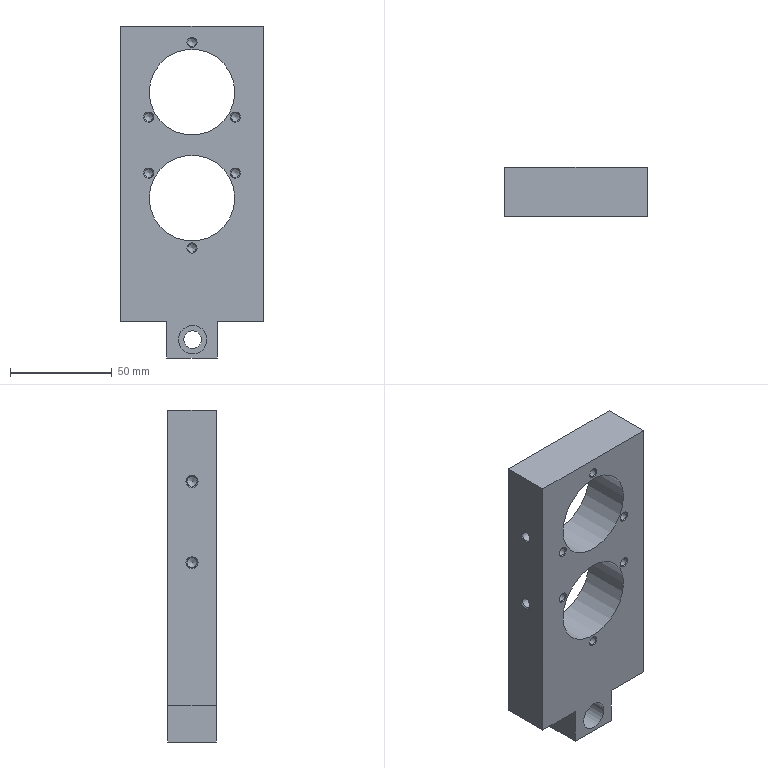Part | STEP file | 冲床-300配套压波_id346_x_t | 1 solid | 45 faces | box 70 x 24 x 163 mm | volume 181383 mm3 | cone 20 | cylinder 14 | plane 11 | commonest cylinder face diameters 4.2 x6 5 x2 8.5 x2 42 x2 8.7 x1 14 x1
STEP:
#1=CARTESIAN_POINT('',(1620.325,-84.,6.65));
#2=VERTEX_POINT('',#1);
#3=CARTESIAN_POINT('',(1620.325,-84.,11.));
#4=DIRECTION('',(0.,-1.,0.));
#5=DIRECTION('',(0.,0.,-1.));
#6=AXIS2_PLACEMENT_3D('',#3,#4,#5);
#7=CIRCLE('',#6,4.35);
#8=EDGE_CURVE('',#2,#2,#7,.T.);
#9=ORIENTED_EDGE('',*,*,#8,.F.);
#10=EDGE_LOOP('',(#9));
#11=FACE_BOUND('',#10,.T.);
#12=CARTESIAN_POINT('',(1620.325,-84.,4.));
#13=VERTEX_POINT('',#12);
#14=CARTESIAN_POINT('',(1620.325,-84.,11.));
#15=DIRECTION('',(0.,-1.,0.));
#16=DIRECTION('',(0.,0.,-1.));
#17=AXIS2_PLACEMENT_3D('',#14,#15,#16);
#18=CIRCLE('',#17,7.);
#19=EDGE_CURVE('',#13,#13,#18,.T.);
#20=ORIENTED_EDGE('',*,*,#19,.T.);
#21=EDGE_LOOP('',(#20));
#22=FACE_BOUND('',#21,.T.);
#23=CARTESIAN_POINT('',(1620.325,-84.,11.));
#24=DIRECTION('',(0.,1.,0.));
#25=DIRECTION('',(0.,0.,-1.));
#26=AXIS2_PLACEMENT_3D('',#23,#24,#25);
#27=PLANE('',#26);
#28=ADVANCED_FACE('',(#11,#22),#27,.F.);
#29=ORIENTED_EDGE('',*,*,#19,.F.);
#30=EDGE_LOOP('',(#29));
#31=FACE_BOUND('',#30,.T.);
#32=CARTESIAN_POINT('',(1620.325,-99.,4.));
#33=VERTEX_POINT('',#32);
#34=CARTESIAN_POINT('',(1620.325,-99.,11.));
#35=DIRECTION('',(0.,1.,0.));
#36=DIRECTION('',(0.,0.,-1.));
#37=AXIS2_PLACEMENT_3D('',#34,#35,#36);
#38=CIRCLE('',#37,7.);
#39=EDGE_CURVE('',#33,#33,#38,.T.);
#40=ORIENTED_EDGE('',*,*,#39,.F.);
#41=EDGE_LOOP('',(#40));
#42=FACE_BOUND('',#41,.T.);
#43=CARTESIAN_POINT('',(1620.325,-99.,11.));
#44=DIRECTION('',(0.,1.,0.));
#45=DIRECTION('',(0.,0.,-1.));
#46=AXIS2_PLACEMENT_3D('',#43,#44,#45);
#47=CYLINDRICAL_SURFACE('',#46,7.);
#48=ADVANCED_FACE('',(#31,#42),#47,.F.);
#49=CARTESIAN_POINT('',(1655.,-75.,165.));
#50=VERTEX_POINT('',#49);
#51=CARTESIAN_POINT('',(1655.,-99.,165.));
#52=VERTEX_POINT('',#51);
#53=CARTESIAN_POINT('',(1655.,-75.,165.));
#54=DIRECTION('',(0.,-1.,0.));
#55=VECTOR('',#54,1.);
#56=LINE('',#53,#55);
#57=EDGE_CURVE('',#50,#52,#56,.T.);
#58=ORIENTED_EDGE('',*,*,#57,.F.);
#59=CARTESIAN_POINT('',(1585.,-75.,165.));
#60=VERTEX_POINT('',#59);
#61=CARTESIAN_POINT('',(1560.,-75.,165.));
#62=DIRECTION('',(1.,0.,0.));
#63=VECTOR('',#62,1.);
#64=LINE('',#61,#63);
#65=EDGE_CURVE('',#60,#50,#64,.T.);
#66=ORIENTED_EDGE('',*,*,#65,.F.);
#67=CARTESIAN_POINT('',(1585.,-99.,165.));
#68=VERTEX_POINT('',#67);
#69=CARTESIAN_POINT('',(1585.,-100.,165.));
#70=DIRECTION('',(0.,1.,0.));
#71=VECTOR('',#70,1.);
#72=LINE('',#69,#71);
#73=EDGE_CURVE('',#68,#60,#72,.T.);
#74=ORIENTED_EDGE('',*,*,#73,.F.);
#75=CARTESIAN_POINT('',(1680.,-99.,165.));
#76=DIRECTION('',(-1.,0.,0.));
#77=VECTOR('',#76,1.);
#78=LINE('',#75,#77);
#79=EDGE_CURVE('',#52,#68,#78,.T.);
#80=ORIENTED_EDGE('',*,*,#79,.F.);
#81=EDGE_LOOP('',(#58,#66,#74,#80));
#82=FACE_OUTER_BOUND('',#81,.T.);
#83=CARTESIAN_POINT('',(1620.,-87.,165.));
#84=DIRECTION('',(0.,0.,-1.));
#85=DIRECTION('',(-1.,0.,0.));
#86=AXIS2_PLACEMENT_3D('',#83,#84,#85);
#87=PLANE('',#86);
#88=ADVANCED_FACE('',(#82),#87,.F.);
#89=CARTESIAN_POINT('',(1655.,-99.,20.));
#90=VERTEX_POINT('',#89);
#91=CARTESIAN_POINT('',(1655.,-99.,170.));
#92=DIRECTION('',(0.,0.,1.));
#93=VECTOR('',#92,1.);
#94=LINE('',#91,#93);
#95=EDGE_CURVE('',#90,#52,#94,.T.);
#96=ORIENTED_EDGE('',*,*,#95,.F.);
#97=CARTESIAN_POINT('',(1655.,-75.,20.));
#98=VERTEX_POINT('',#97);
#99=CARTESIAN_POINT('',(1655.,-75.,20.));
#100=DIRECTION('',(0.,1.,0.));
#101=VECTOR('',#100,1.);
#102=LINE('',#99,#101);
#103=EDGE_CURVE('',#90,#98,#102,.T.);
#104=ORIENTED_EDGE('',*,*,#103,.T.);
#105=CARTESIAN_POINT('',(1655.,-75.,170.));
#106=DIRECTION('',(0.,0.,1.));
#107=VECTOR('',#106,1.);
#108=LINE('',#105,#107);
#109=EDGE_CURVE('',#98,#50,#108,.T.);
#110=ORIENTED_EDGE('',*,*,#109,.T.);
#111=ORIENTED_EDGE('',*,*,#57,.T.);
#112=EDGE_LOOP('',(#96,#104,#110,#111));
#113=FACE_OUTER_BOUND('',#112,.T.);
#114=CARTESIAN_POINT('',(1655.,-75.,170.));
#115=DIRECTION('',(-1.,0.,0.));
#116=DIRECTION('',(0.,0.,1.));
#117=AXIS2_PLACEMENT_3D('',#114,#115,#116);
#118=PLANE('',#117);
#119=ADVANCED_FACE('',(#113),#118,.F.);
#120=CARTESIAN_POINT('',(1650.,-87.,20.));
#121=VERTEX_POINT('',#120);
#122=CARTESIAN_POINT('',(1645.,-87.,20.));
#123=DIRECTION('',(0.,0.,1.));
#124=DIRECTION('',(1.,0.,0.));
#125=AXIS2_PLACEMENT_3D('',#122,#123,#124);
#126=CIRCLE('',#125,5.);
#127=EDGE_CURVE('',#121,#121,#126,.T.);
#128=ORIENTED_EDGE('',*,*,#127,.T.);
#129=EDGE_LOOP('',(#128));
#130=FACE_BOUND('',#129,.T.);
#131=CARTESIAN_POINT('',(1632.5,-75.,20.));
#132=VERTEX_POINT('',#131);
#133=CARTESIAN_POINT('',(1560.,-75.,20.));
#134=DIRECTION('',(-1.,0.,0.));
#135=VECTOR('',#134,1.);
#136=LINE('',#133,#135);
#137=EDGE_CURVE('',#98,#132,#136,.T.);
#138=ORIENTED_EDGE('',*,*,#137,.F.);
#139=ORIENTED_EDGE('',*,*,#103,.F.);
#140=CARTESIAN_POINT('',(1632.5,-99.,20.));
#141=VERTEX_POINT('',#140);
#142=CARTESIAN_POINT('',(1680.,-99.,20.));
#143=DIRECTION('',(1.,0.,0.));
#144=VECTOR('',#143,1.);
#145=LINE('',#142,#144);
#146=EDGE_CURVE('',#141,#90,#145,.T.);
#147=ORIENTED_EDGE('',*,*,#146,.F.);
#148=CARTESIAN_POINT('',(1632.5,0.,20.));
#149=DIRECTION('',(0.,1.,0.));
#150=VECTOR('',#149,1.);
#151=LINE('',#148,#150);
#152=EDGE_CURVE('',#141,#132,#151,.T.);
#153=ORIENTED_EDGE('',*,*,#152,.T.);
#154=EDGE_LOOP('',(#138,#139,#147,#153));
#155=FACE_BOUND('',#154,.T.);
#156=CARTESIAN_POINT('',(1660.,0.,20.));
#157=DIRECTION('',(0.,0.,1.));
#158=DIRECTION('',(1.,0.,0.));
#159=AXIS2_PLACEMENT_3D('',#156,#157,#158);
#160=PLANE('',#159);
#161=ADVANCED_FACE('',(#130,#155),#160,.F.);
#162=ORIENTED_EDGE('',*,*,#152,.F.);
#163=CARTESIAN_POINT('',(1632.5,-99.,2.));
#164=VERTEX_POINT('',#163);
#165=CARTESIAN_POINT('',(1632.5,-99.,37.685));
#166=DIRECTION('',(0.,0.,1.));
#167=VECTOR('',#166,1.);
#168=LINE('',#165,#167);
#169=EDGE_CURVE('',#164,#141,#168,.T.);
#170=ORIENTED_EDGE('',*,*,#169,.F.);
#171=CARTESIAN_POINT('',(1632.5,-75.,2.));
#172=VERTEX_POINT('',#171);
#173=CARTESIAN_POINT('',(1632.5,-75.,2.));
#174=DIRECTION('',(0.,1.,0.));
#175=VECTOR('',#174,1.);
#176=LINE('',#173,#175);
#177=EDGE_CURVE('',#164,#172,#176,.T.);
#178=ORIENTED_EDGE('',*,*,#177,.T.);
#179=CARTESIAN_POINT('',(1632.5,-75.,37.685));
#180=DIRECTION('',(0.,0.,1.));
#181=VECTOR('',#180,1.);
#182=LINE('',#179,#181);
#183=EDGE_CURVE('',#172,#132,#182,.T.);
#184=ORIENTED_EDGE('',*,*,#183,.T.);
#185=EDGE_LOOP('',(#162,#170,#178,#184));
#186=FACE_OUTER_BOUND('',#185,.T.);
#187=CARTESIAN_POINT('',(1632.5,-75.,37.685));
#188=DIRECTION('',(1.,0.,0.));
#189=DIRECTION('',(0.,0.,-1.));
#190=AXIS2_PLACEMENT_3D('',#187,#188,#189);
#191=PLANE('',#190);
#192=ADVANCED_FACE('',(#186),#191,.T.);
#193=CARTESIAN_POINT('',(1607.5,-99.,2.));
#194=VERTEX_POINT('',#193);
#195=CARTESIAN_POINT('',(1660.,-99.,2.));
#196=DIRECTION('',(1.,0.,0.));
#197=VECTOR('',#196,1.);
#198=LINE('',#195,#197);
#199=EDGE_CURVE('',#194,#164,#198,.T.);
#200=ORIENTED_EDGE('',*,*,#199,.F.);
#201=CARTESIAN_POINT('',(1607.5,-75.,2.));
#202=VERTEX_POINT('',#201);
#203=CARTESIAN_POINT('',(1607.5,0.,2.));
#204=DIRECTION('',(0.,1.,0.));
#205=VECTOR('',#204,1.);
#206=LINE('',#203,#205);
#207=EDGE_CURVE('',#194,#202,#206,.T.);
#208=ORIENTED_EDGE('',*,*,#207,.T.);
#209=CARTESIAN_POINT('',(1560.,-75.,2.));
#210=DIRECTION('',(1.,0.,0.));
#211=VECTOR('',#210,1.);
#212=LINE('',#209,#211);
#213=EDGE_CURVE('',#202,#172,#212,.T.);
#214=ORIENTED_EDGE('',*,*,#213,.T.);
#215=ORIENTED_EDGE('',*,*,#177,.F.);
#216=EDGE_LOOP('',(#200,#208,#214,#215));
#217=FACE_OUTER_BOUND('',#216,.T.);
#218=CARTESIAN_POINT('',(1660.,0.,2.));
#219=DIRECTION('',(0.,0.,1.));
#220=DIRECTION('',(1.,0.,0.));
#221=AXIS2_PLACEMENT_3D('',#218,#219,#220);
#222=PLANE('',#221);
#223=ADVANCED_FACE('',(#217),#222,.F.);
#224=CARTESIAN_POINT('',(1607.5,-75.,20.));
#225=VERTEX_POINT('',#224);
#226=CARTESIAN_POINT('',(1607.5,-99.,20.));
#227=VERTEX_POINT('',#226);
#228=CARTESIAN_POINT('',(1607.5,0.,20.));
#229=DIRECTION('',(0.,-1.,0.));
#230=VECTOR('',#229,1.);
#231=LINE('',#228,#230);
#232=EDGE_CURVE('',#225,#227,#231,.T.);
#233=ORIENTED_EDGE('',*,*,#232,.F.);
#234=CARTESIAN_POINT('',(1607.5,-75.,-18.315));
#235=DIRECTION('',(0.,0.,-1.));
#236=VECTOR('',#235,1.);
#237=LINE('',#234,#236);
#238=EDGE_CURVE('',#225,#202,#237,.T.);
#239=ORIENTED_EDGE('',*,*,#238,.T.);
#240=ORIENTED_EDGE('',*,*,#207,.F.);
#241=CARTESIAN_POINT('',(1607.5,-99.,-18.315));
#242=DIRECTION('',(0.,0.,-1.));
#243=VECTOR('',#242,1.);
#244=LINE('',#241,#243);
#245=EDGE_CURVE('',#227,#194,#244,.T.);
#246=ORIENTED_EDGE('',*,*,#245,.F.);
#247=EDGE_LOOP('',(#233,#239,#240,#246));
#248=FACE_OUTER_BOUND('',#247,.T.);
#249=CARTESIAN_POINT('',(1607.5,-75.,-18.315));
#250=DIRECTION('',(-1.,0.,0.));
#251=DIRECTION('',(0.,0.,1.));
#252=AXIS2_PLACEMENT_3D('',#249,#250,#251);
#253=PLANE('',#252);
#254=ADVANCED_FACE('',(#248),#253,.T.);
#255=CARTESIAN_POINT('',(1600.,-87.,20.));
#256=VERTEX_POINT('',#255);
#257=CARTESIAN_POINT('',(1595.,-87.,20.));
#258=DIRECTION('',(0.,0.,1.));
#259=DIRECTION('',(1.,0.,0.));
#260=AXIS2_PLACEMENT_3D('',#257,#258,#259);
#261=CIRCLE('',#260,5.);
#262=EDGE_CURVE('',#256,#256,#261,.T.);
#263=ORIENTED_EDGE('',*,*,#262,.T.);
#264=EDGE_LOOP('',(#263));
#265=FACE_BOUND('',#264,.T.);
#266=CARTESIAN_POINT('',(1585.,-99.,20.));
#267=VERTEX_POINT('',#266);
#268=CARTESIAN_POINT('',(1680.,-99.,20.));
#269=DIRECTION('',(1.,0.,0.));
#270=VECTOR('',#269,1.);
#271=LINE('',#268,#270);
#272=EDGE_CURVE('',#267,#227,#271,.T.);
#273=ORIENTED_EDGE('',*,*,#272,.F.);
#274=CARTESIAN_POINT('',(1585.,-75.,20.));
#275=VERTEX_POINT('',#274);
#276=CARTESIAN_POINT('',(1585.,-100.,20.));
#277=DIRECTION('',(0.,-1.,0.));
#278=VECTOR('',#277,1.);
#279=LINE('',#276,#278);
#280=EDGE_CURVE('',#275,#267,#279,.T.);
#281=ORIENTED_EDGE('',*,*,#280,.F.);
#282=CARTESIAN_POINT('',(1560.,-75.,20.));
#283=DIRECTION('',(-1.,0.,0.));
#284=VECTOR('',#283,1.);
#285=LINE('',#282,#284);
#286=EDGE_CURVE('',#225,#275,#285,.T.);
#287=ORIENTED_EDGE('',*,*,#286,.F.);
#288=ORIENTED_EDGE('',*,*,#232,.T.);
#289=EDGE_LOOP('',(#273,#281,#287,#288));
#290=FACE_BOUND('',#289,.T.);
#291=CARTESIAN_POINT('',(1660.,0.,20.));
#292=DIRECTION('',(0.,0.,1.));
#293=DIRECTION('',(1.,0.,0.));
#294=AXIS2_PLACEMENT_3D('',#291,#292,#293);
#295=PLANE('',#294);
#296=ADVANCED_FACE('',(#265,#290),#295,.F.);
#297=ORIENTED_EDGE('',*,*,#8,.T.);
#298=EDGE_LOOP('',(#297));
#299=FACE_BOUND('',#298,.T.);
#300=CARTESIAN_POINT('',(1615.975,-75.,11.));
#301=VERTEX_POINT('',#300);
#302=CARTESIAN_POINT('',(1620.325,-75.,11.));
#303=DIRECTION('',(0.,-1.,0.));
#304=DIRECTION('',(-1.,0.,0.));
#305=AXIS2_PLACEMENT_3D('',#302,#303,#304);
#306=CIRCLE('',#305,4.35);
#307=EDGE_CURVE('',#301,#301,#306,.T.);
#308=ORIENTED_EDGE('',*,*,#307,.F.);
#309=EDGE_LOOP('',(#308));
#310=FACE_BOUND('',#309,.T.);
#311=CARTESIAN_POINT('',(1620.325,-49.,11.));
#312=DIRECTION('',(0.,1.,0.));
#313=DIRECTION('',(0.,0.,-1.));
#314=AXIS2_PLACEMENT_3D('',#311,#312,#313);
#315=CYLINDRICAL_SURFACE('',#314,4.35);
#316=ADVANCED_FACE('',(#299,#310),#315,.F.);
#317=CARTESIAN_POINT('',(1638.718,-99.,92.75));
#318=VERTEX_POINT('',#317);
#319=CARTESIAN_POINT('',(1641.218,-99.,92.75));
#320=DIRECTION('',(0.,1.,0.));
#321=DIRECTION('',(-1.,0.,0.));
#322=AXIS2_PLACEMENT_3D('',#319,#320,#321);
#323=CIRCLE('',#322,2.5);
#324=EDGE_CURVE('',#318,#318,#323,.T.);
#325=ORIENTED_EDGE('',*,*,#324,.T.);
#326=EDGE_LOOP('',(#325));
#327=FACE_BOUND('',#326,.T.);
#328=CARTESIAN_POINT('',(1617.5,-99.,56.));
#329=VERTEX_POINT('',#328);
#330=CARTESIAN_POINT('',(1620.,-99.,56.));
#331=DIRECTION('',(0.,1.,0.));
#332=DIRECTION('',(-1.,0.,0.));
#333=AXIS2_PLACEMENT_3D('',#330,#331,#332);
#334=CIRCLE('',#333,2.5);
#335=EDGE_CURVE('',#329,#329,#334,.T.);
#336=ORIENTED_EDGE('',*,*,#335,.T.);
#337=EDGE_LOOP('',(#336));
#338=FACE_BOUND('',#337,.T.);
#339=CARTESIAN_POINT('',(1596.282,-99.,92.75));
#340=VERTEX_POINT('',#339);
#341=CARTESIAN_POINT('',(1598.782,-99.,92.75));
#342=DIRECTION('',(0.,1.,0.));
#343=DIRECTION('',(-1.,0.,0.));
#344=AXIS2_PLACEMENT_3D('',#341,#342,#343);
#345=CIRCLE('',#344,2.5);
#346=EDGE_CURVE('',#340,#340,#345,.T.);
#347=ORIENTED_EDGE('',*,*,#346,.T.);
#348=EDGE_LOOP('',(#347));
#349=FACE_BOUND('',#348,.T.);
#350=CARTESIAN_POINT('',(1638.718,-99.,120.25));
#351=VERTEX_POINT('',#350);
#352=CARTESIAN_POINT('',(1641.218,-99.,120.25));
#353=DIRECTION('',(0.,1.,0.));
#354=DIRECTION('',(-1.,0.,0.));
#355=AXIS2_PLACEMENT_3D('',#352,#353,#354);
#356=CIRCLE('',#355,2.5);
#357=EDGE_CURVE('',#351,#351,#356,.T.);
#358=ORIENTED_EDGE('',*,*,#357,.T.);
#359=EDGE_LOOP('',(#358));
#360=FACE_BOUND('',#359,.T.);
#361=CARTESIAN_POINT('',(1596.282,-99.,120.25));
#362=VERTEX_POINT('',#361);
#363=CARTESIAN_POINT('',(1598.782,-99.,120.25));
#364=DIRECTION('',(0.,1.,0.));
#365=DIRECTION('',(-1.,0.,0.));
#366=AXIS2_PLACEMENT_3D('',#363,#364,#365);
#367=CIRCLE('',#366,2.5);
#368=EDGE_CURVE('',#362,#362,#367,.T.);
#369=ORIENTED_EDGE('',*,*,#368,.T.);
#370=EDGE_LOOP('',(#369));
#371=FACE_BOUND('',#370,.T.);
#372=CARTESIAN_POINT('',(1617.5,-99.,157.));
#373=VERTEX_POINT('',#372);
#374=CARTESIAN_POINT('',(1620.,-99.,157.));
#375=DIRECTION('',(0.,1.,0.));
#376=DIRECTION('',(-1.,0.,0.));
#377=AXIS2_PLACEMENT_3D('',#374,#375,#376);
#378=CIRCLE('',#377,2.5);
#379=EDGE_CURVE('',#373,#373,#378,.T.);
#380=ORIENTED_EDGE('',*,*,#379,.T.);
#381=EDGE_LOOP('',(#380));
#382=FACE_BOUND('',#381,.T.);
#383=CARTESIAN_POINT('',(1599.,-99.,80.5));
#384=VERTEX_POINT('',#383);
#385=CARTESIAN_POINT('',(1620.,-99.,80.5));
#386=DIRECTION('',(0.,1.,0.));
#387=DIRECTION('',(-1.,0.,0.));
#388=AXIS2_PLACEMENT_3D('',#385,#386,#387);
#389=CIRCLE('',#388,21.);
#390=EDGE_CURVE('',#384,#384,#389,.T.);
#391=ORIENTED_EDGE('',*,*,#390,.T.);
#392=EDGE_LOOP('',(#391));
#393=FACE_BOUND('',#392,.T.);
#394=CARTESIAN_POINT('',(1599.,-99.,132.5));
#395=VERTEX_POINT('',#394);
#396=CARTESIAN_POINT('',(1620.,-99.,132.5));
#397=DIRECTION('',(0.,1.,0.));
#398=DIRECTION('',(-1.,0.,0.));
#399=AXIS2_PLACEMENT_3D('',#396,#397,#398);
#400=CIRCLE('',#399,21.);
#401=EDGE_CURVE('',#395,#395,#400,.T.);
#402=ORIENTED_EDGE('',*,*,#401,.T.);
#403=EDGE_LOOP('',(#402));
#404=FACE_BOUND('',#403,.T.);
#405=CARTESIAN_POINT('',(1585.,-99.,170.));
#406=DIRECTION('',(0.,0.,1.));
#407=VECTOR('',#406,1.);
#408=LINE('',#405,#407);
#409=EDGE_CURVE('',#267,#68,#408,.T.);
#410=ORIENTED_EDGE('',*,*,#409,.F.);
#411=ORIENTED_EDGE('',*,*,#272,.T.);
#412=ORIENTED_EDGE('',*,*,#245,.T.);
#413=ORIENTED_EDGE('',*,*,#199,.T.);
#414=ORIENTED_EDGE('',*,*,#169,.T.);
#415=ORIENTED_EDGE('',*,*,#146,.T.);
#416=ORIENTED_EDGE('',*,*,#95,.T.);
#417=ORIENTED_EDGE('',*,*,#79,.T.);
#418=EDGE_LOOP('',(#410,#411,#412,#413,#414,#415,#416,#417));
#419=FACE_BOUND('',#418,.T.);
#420=ORIENTED_EDGE('',*,*,#39,.T.);
#421=EDGE_LOOP('',(#420));
#422=FACE_BOUND('',#421,.T.);
#423=CARTESIAN_POINT('',(1680.,-99.,170.));
#424=DIRECTION('',(0.,1.,0.));
#425=DIRECTION('',(0.,0.,-1.));
#426=AXIS2_PLACEMENT_3D('',#423,#424,#425);
#427=PLANE('',#426);
#428=ADVANCED_FACE('',(#327,#338,#349,#360,#371,#382,#393,#404,#419,#422),#427,.F.);
#429=CARTESIAN_POINT('',(1641.,-75.,80.5));
#430=VERTEX_POINT('',#429);
#431=CARTESIAN_POINT('',(1620.,-75.,80.5));
#432=DIRECTION('',(0.,-1.,0.));
#433=DIRECTION('',(1.,0.,0.));
#434=AXIS2_PLACEMENT_3D('',#431,#432,#433);
#435=CIRCLE('',#434,21.);
#436=EDGE_CURVE('',#430,#430,#435,.T.);
#437=ORIENTED_EDGE('',*,*,#436,.T.);
#438=EDGE_LOOP('',(#437));
#439=FACE_BOUND('',#438,.T.);
#440=CARTESIAN_POINT('',(1641.,-75.,132.5));
#441=VERTEX_POINT('',#440);
#442=CARTESIAN_POINT('',(1620.,-75.,132.5));
#443=DIRECTION('',(0.,-1.,0.));
#444=DIRECTION('',(1.,0.,0.));
#445=AXIS2_PLACEMENT_3D('',#442,#443,#444);
#446=CIRCLE('',#445,21.);
#447=EDGE_CURVE('',#441,#441,#446,.T.);
#448=ORIENTED_EDGE('',*,*,#447,.T.);
#449=EDGE_LOOP('',(#448));
#450=FACE_BOUND('',#449,.T.);
#451=CARTESIAN_POINT('',(1585.,-75.,170.));
#452=DIRECTION('',(0.,0.,1.));
#453=VECTOR('',#452,1.);
#454=LINE('',#451,#453);
#455=EDGE_CURVE('',#275,#60,#454,.T.);
#456=ORIENTED_EDGE('',*,*,#455,.T.);
#457=ORIENTED_EDGE('',*,*,#65,.T.);
#458=ORIENTED_EDGE('',*,*,#109,.F.);
#459=ORIENTED_EDGE('',*,*,#137,.T.);
#460=ORIENTED_EDGE('',*,*,#183,.F.);
#461=ORIENTED_EDGE('',*,*,#213,.F.);
#462=ORIENTED_EDGE('',*,*,#238,.F.);
#463=ORIENTED_EDGE('',*,*,#286,.T.);
#464=EDGE_LOOP('',(#456,#457,#458,#459,#460,#461,#462,#463));
#465=FACE_BOUND('',#464,.T.);
#466=ORIENTED_EDGE('',*,*,#307,.T.);
#467=EDGE_LOOP('',(#466));
#468=FACE_BOUND('',#467,.T.);
#469=CARTESIAN_POINT('',(1560.,-75.,170.));
#470=DIRECTION('',(0.,-1.,0.));
#471=DIRECTION('',(-1.,0.,0.));
#472=AXIS2_PLACEMENT_3D('',#469,#470,#471);
#473=PLANE('',#472);
#474=ADVANCED_FACE('',(#439,#450,#465,#468),#473,.F.);
#475=CARTESIAN_POINT('',(1585.,-90.,130.));
#476=VERTEX_POINT('',#475);
#477=CARTESIAN_POINT('',(1585.,-87.,130.));
#478=DIRECTION('',(1.,0.,0.));
#479=DIRECTION('',(0.,-1.,0.));
#480=AXIS2_PLACEMENT_3D('',#477,#478,#479);
#481=CIRCLE('',#480,3.);
#482=EDGE_CURVE('',#476,#476,#481,.T.);
#483=ORIENTED_EDGE('',*,*,#482,.T.);
#484=EDGE_LOOP('',(#483));
#485=FACE_BOUND('',#484,.T.);
#486=CARTESIAN_POINT('',(1585.,-90.,90.));
#487=VERTEX_POINT('',#486);
#488=CARTESIAN_POINT('',(1585.,-87.,90.));
#489=DIRECTION('',(1.,0.,0.));
#490=DIRECTION('',(0.,-1.,0.));
#491=AXIS2_PLACEMENT_3D('',#488,#489,#490);
#492=CIRCLE('',#491,3.);
#493=EDGE_CURVE('',#487,#487,#492,.T.);
#494=ORIENTED_EDGE('',*,*,#493,.T.);
#495=EDGE_LOOP('',(#494));
#496=FACE_BOUND('',#495,.T.);
#497=ORIENTED_EDGE('',*,*,#409,.T.);
#498=ORIENTED_EDGE('',*,*,#73,.T.);
#499=ORIENTED_EDGE('',*,*,#455,.F.);
#500=ORIENTED_EDGE('',*,*,#280,.T.);
#501=EDGE_LOOP('',(#497,#498,#499,#500));
#502=FACE_BOUND('',#501,.T.);
#503=CARTESIAN_POINT('',(1585.,-100.,170.));
#504=DIRECTION('',(1.,0.,0.));
#505=DIRECTION('',(0.,0.,-1.));
#506=AXIS2_PLACEMENT_3D('',#503,#504,#505);
#507=PLANE('',#506);
#508=ADVANCED_FACE('',(#485,#496,#502),#507,.F.);
#509=ORIENTED_EDGE('',*,*,#447,.F.);
#510=EDGE_LOOP('',(#509));
#511=FACE_BOUND('',#510,.T.);
#512=ORIENTED_EDGE('',*,*,#401,.F.);
#513=EDGE_LOOP('',(#512));
#514=FACE_BOUND('',#513,.T.);
#515=CARTESIAN_POINT('',(1620.,-225.9,132.5));
#516=DIRECTION('',(0.,1.,0.));
#517=DIRECTION('',(-1.,0.,0.));
#518=AXIS2_PLACEMENT_3D('',#515,#516,#517);
#519=CYLINDRICAL_SURFACE('',#518,21.);
#520=ADVANCED_FACE('',(#511,#514),#519,.F.);
#521=ORIENTED_EDGE('',*,*,#436,.F.);
#522=EDGE_LOOP('',(#521));
#523=FACE_BOUND('',#522,.T.);
#524=ORIENTED_EDGE('',*,*,#390,.F.);
#525=EDGE_LOOP('',(#524));
#526=FACE_BOUND('',#525,.T.);
#527=CARTESIAN_POINT('',(1620.,-225.9,80.5));
#528=DIRECTION('',(0.,1.,0.));
#529=DIRECTION('',(-1.,0.,0.));
#530=AXIS2_PLACEMENT_3D('',#527,#528,#529);
#531=CYLINDRICAL_SURFACE('',#530,21.);
#532=ADVANCED_FACE('',(#523,#526),#531,.F.);
#533=CARTESIAN_POINT('',(1599.25,-87.,40.));
#534=VERTEX_POINT('',#533);
#535=CARTESIAN_POINT('',(1595.,-87.,40.));
#536=DIRECTION('',(0.,0.,-1.));
#537=DIRECTION('',(1.,0.,0.));
#538=AXIS2_PLACEMENT_3D('',#535,#536,#537);
#539=CIRCLE('',#538,4.25);
#540=EDGE_CURVE('',#534,#534,#539,.T.);
#541=ORIENTED_EDGE('',*,*,#540,.T.);
#542=EDGE_LOOP('',(#541));
#543=FACE_BOUND('',#542,.T.);
#544=CARTESIAN_POINT('',(1595.,-87.,42.554));
#545=VERTEX_POINT('',#544);
#546=VERTEX_LOOP('',#545);
#547=FACE_BOUND('',#546,.T.);
#548=CARTESIAN_POINT('',(1595.,-87.,40.));
#549=DIRECTION('',(0.,0.,-1.));
#550=DIRECTION('',(-1.,0.,0.));
#551=AXIS2_PLACEMENT_3D('',#548,#549,#550);
#552=CONICAL_SURFACE('',#551,4.25,59.);
#553=ADVANCED_FACE('',(#543,#547),#552,.F.);
#554=CARTESIAN_POINT('',(1599.25,-87.,20.75));
#555=VERTEX_POINT('',#554);
#556=CARTESIAN_POINT('',(1595.,-87.,20.75));
#557=DIRECTION('',(0.,0.,-1.));
#558=DIRECTION('',(1.,0.,0.));
#559=AXIS2_PLACEMENT_3D('',#556,#557,#558);
#560=CIRCLE('',#559,4.25);
#561=EDGE_CURVE('',#555,#555,#560,.T.);
#562=ORIENTED_EDGE('',*,*,#561,.T.);
#563=EDGE_LOOP('',(#562));
#564=FACE_BOUND('',#563,.T.);
#565=ORIENTED_EDGE('',*,*,#540,.F.);
#566=EDGE_LOOP('',(#565));
#567=FACE_BOUND('',#566,.T.);
#568=CARTESIAN_POINT('',(1595.,-87.,20.));
#569=DIRECTION('',(0.,0.,1.));
#570=DIRECTION('',(1.,0.,0.));
#571=AXIS2_PLACEMENT_3D('',#568,#569,#570);
#572=CYLINDRICAL_SURFACE('',#571,4.25);
#573=ADVANCED_FACE('',(#564,#567),#572,.F.);
#574=ORIENTED_EDGE('',*,*,#561,.F.);
#575=EDGE_LOOP('',(#574));
#576=FACE_BOUND('',#575,.T.);
#577=ORIENTED_EDGE('',*,*,#262,.F.);
#578=EDGE_LOOP('',(#577));
#579=FACE_BOUND('',#578,.T.);
#580=CARTESIAN_POINT('',(1595.,-87.,20.));
#581=DIRECTION('',(0.,0.,-1.));
#582=DIRECTION('',(-1.,0.,0.));
#583=AXIS2_PLACEMENT_3D('',#580,#581,#582);
#584=CONICAL_SURFACE('',#583,5.,45.);
#585=ADVANCED_FACE('',(#576,#579),#584,.F.);
#586=CARTESIAN_POINT('',(1649.25,-87.,40.));
#587=VERTEX_POINT('',#586);
#588=CARTESIAN_POINT('',(1645.,-87.,40.));
#589=DIRECTION('',(0.,0.,-1.));
#590=DIRECTION('',(1.,0.,0.));
#591=AXIS2_PLACEMENT_3D('',#588,#589,#590);
#592=CIRCLE('',#591,4.25);
#593=EDGE_CURVE('',#587,#587,#592,.T.);
#594=ORIENTED_EDGE('',*,*,#593,.T.);
#595=EDGE_LOOP('',(#594));
#596=FACE_BOUND('',#595,.T.);
#597=CARTESIAN_POINT('',(1645.,-87.,42.554));
#598=VERTEX_POINT('',#597);
#599=VERTEX_LOOP('',#598);
#600=FACE_BOUND('',#599,.T.);
#601=CARTESIAN_POINT('',(1645.,-87.,40.));
#602=DIRECTION('',(0.,0.,-1.));
#603=DIRECTION('',(-1.,0.,0.));
#604=AXIS2_PLACEMENT_3D('',#601,#602,#603);
#605=CONICAL_SURFACE('',#604,4.25,59.);
#606=ADVANCED_FACE('',(#596,#600),#605,.F.);
#607=CARTESIAN_POINT('',(1649.25,-87.,20.75));
#608=VERTEX_POINT('',#607);
#609=CARTESIAN_POINT('',(1645.,-87.,20.75));
#610=DIRECTION('',(0.,0.,-1.));
#611=DIRECTION('',(1.,0.,0.));
#612=AXIS2_PLACEMENT_3D('',#609,#610,#611);
#613=CIRCLE('',#612,4.25);
#614=EDGE_CURVE('',#608,#608,#613,.T.);
#615=ORIENTED_EDGE('',*,*,#614,.T.);
#616=EDGE_LOOP('',(#615));
#617=FACE_BOUND('',#616,.T.);
#618=ORIENTED_EDGE('',*,*,#593,.F.);
#619=EDGE_LOOP('',(#618));
#620=FACE_BOUND('',#619,.T.);
#621=CARTESIAN_POINT('',(1645.,-87.,20.));
#622=DIRECTION('',(0.,0.,1.));
#623=DIRECTION('',(1.,0.,0.));
#624=AXIS2_PLACEMENT_3D('',#621,#622,#623);
#625=CYLINDRICAL_SURFACE('',#624,4.25);
#626=ADVANCED_FACE('',(#617,#620),#625,.F.);
#627=ORIENTED_EDGE('',*,*,#614,.F.);
#628=EDGE_LOOP('',(#627));
#629=FACE_BOUND('',#628,.T.);
#630=ORIENTED_EDGE('',*,*,#127,.F.);
#631=EDGE_LOOP('',(#630));
#632=FACE_BOUND('',#631,.T.);
#633=CARTESIAN_POINT('',(1645.,-87.,20.));
#634=DIRECTION('',(0.,0.,-1.));
#635=DIRECTION('',(-1.,0.,0.));
#636=AXIS2_PLACEMENT_3D('',#633,#634,#635);
#637=CONICAL_SURFACE('',#636,5.,45.);
#638=ADVANCED_FACE('',(#629,#632),#637,.F.);
#639=CARTESIAN_POINT('',(1595.,-89.5,90.));
#640=VERTEX_POINT('',#639);
#641=CARTESIAN_POINT('',(1595.,-87.,90.));
#642=DIRECTION('',(-1.,0.,0.));
#643=DIRECTION('',(0.,-1.,0.));
#644=AXIS2_PLACEMENT_3D('',#641,#642,#643);
#645=CIRCLE('',#644,2.5);
#646=EDGE_CURVE('',#640,#640,#645,.T.);
#647=ORIENTED_EDGE('',*,*,#646,.T.);
#648=EDGE_LOOP('',(#647));
#649=FACE_BOUND('',#648,.T.);
#650=CARTESIAN_POINT('',(1596.502,-87.,90.));
#651=VERTEX_POINT('',#650);
#652=VERTEX_LOOP('',#651);
#653=FACE_BOUND('',#652,.T.);
#654=CARTESIAN_POINT('',(1595.,-87.,90.));
#655=DIRECTION('',(-1.,0.,0.));
#656=DIRECTION('',(0.,1.,0.));
#657=AXIS2_PLACEMENT_3D('',#654,#655,#656);
#658=CONICAL_SURFACE('',#657,2.5,59.);
#659=ADVANCED_FACE('',(#649,#653),#658,.F.);
#660=CARTESIAN_POINT('',(1585.5,-87.,87.5));
#661=VERTEX_POINT('',#660);
#662=CARTESIAN_POINT('',(1585.5,-87.,90.));
#663=DIRECTION('',(-1.,0.,0.));
#664=DIRECTION('',(0.,0.,-1.));
#665=AXIS2_PLACEMENT_3D('',#662,#663,#664);
#666=CIRCLE('',#665,2.5);
#667=EDGE_CURVE('',#661,#661,#666,.T.);
#668=ORIENTED_EDGE('',*,*,#667,.T.);
#669=EDGE_LOOP('',(#668));
#670=FACE_BOUND('',#669,.T.);
#671=ORIENTED_EDGE('',*,*,#646,.F.);
#672=EDGE_LOOP('',(#671));
#673=FACE_BOUND('',#672,.T.);
#674=CARTESIAN_POINT('',(1585.,-87.,90.));
#675=DIRECTION('',(1.,0.,0.));
#676=DIRECTION('',(0.,-1.,0.));
#677=AXIS2_PLACEMENT_3D('',#674,#675,#676);
#678=CYLINDRICAL_SURFACE('',#677,2.5);
#679=ADVANCED_FACE('',(#670,#673),#678,.F.);
#680=ORIENTED_EDGE('',*,*,#667,.F.);
#681=EDGE_LOOP('',(#680));
#682=FACE_BOUND('',#681,.T.);
#683=ORIENTED_EDGE('',*,*,#493,.F.);
#684=EDGE_LOOP('',(#683));
#685=FACE_BOUND('',#684,.T.);
#686=CARTESIAN_POINT('',(1585.,-87.,90.));
#687=DIRECTION('',(-1.,0.,0.));
#688=DIRECTION('',(0.,0.,1.));
#689=AXIS2_PLACEMENT_3D('',#686,#687,#688);
#690=CONICAL_SURFACE('',#689,3.,45.);
#691=ADVANCED_FACE('',(#682,#685),#690,.F.);
#692=CARTESIAN_POINT('',(1595.,-89.5,130.));
#693=VERTEX_POINT('',#692);
#694=CARTESIAN_POINT('',(1595.,-87.,130.));
#695=DIRECTION('',(-1.,0.,0.));
#696=DIRECTION('',(0.,-1.,0.));
#697=AXIS2_PLACEMENT_3D('',#694,#695,#696);
#698=CIRCLE('',#697,2.5);
#699=EDGE_CURVE('',#693,#693,#698,.T.);
#700=ORIENTED_EDGE('',*,*,#699,.T.);
#701=EDGE_LOOP('',(#700));
#702=FACE_BOUND('',#701,.T.);
#703=CARTESIAN_POINT('',(1596.502,-87.,130.));
#704=VERTEX_POINT('',#703);
#705=VERTEX_LOOP('',#704);
#706=FACE_BOUND('',#705,.T.);
#707=CARTESIAN_POINT('',(1595.,-87.,130.));
#708=DIRECTION('',(-1.,0.,0.));
#709=DIRECTION('',(0.,1.,0.));
#710=AXIS2_PLACEMENT_3D('',#707,#708,#709);
#711=CONICAL_SURFACE('',#710,2.5,59.);
#712=ADVANCED_FACE('',(#702,#706),#711,.F.);
#713=CARTESIAN_POINT('',(1585.5,-87.,127.5));
#714=VERTEX_POINT('',#713);
#715=CARTESIAN_POINT('',(1585.5,-87.,130.));
#716=DIRECTION('',(-1.,0.,0.));
#717=DIRECTION('',(0.,0.,-1.));
#718=AXIS2_PLACEMENT_3D('',#715,#716,#717);
#719=CIRCLE('',#718,2.5);
#720=EDGE_CURVE('',#714,#714,#719,.T.);
#721=ORIENTED_EDGE('',*,*,#720,.T.);
#722=EDGE_LOOP('',(#721));
#723=FACE_BOUND('',#722,.T.);
#724=ORIENTED_EDGE('',*,*,#699,.F.);
#725=EDGE_LOOP('',(#724));
#726=FACE_BOUND('',#725,.T.);
#727=CARTESIAN_POINT('',(1585.,-87.,130.));
#728=DIRECTION('',(1.,0.,0.));
#729=DIRECTION('',(0.,-1.,0.));
#730=AXIS2_PLACEMENT_3D('',#727,#728,#729);
#731=CYLINDRICAL_SURFACE('',#730,2.5);
#732=ADVANCED_FACE('',(#723,#726),#731,.F.);
#733=ORIENTED_EDGE('',*,*,#720,.F.);
#734=EDGE_LOOP('',(#733));
#735=FACE_BOUND('',#734,.T.);
#736=ORIENTED_EDGE('',*,*,#482,.F.);
#737=EDGE_LOOP('',(#736));
#738=FACE_BOUND('',#737,.T.);
#739=CARTESIAN_POINT('',(1585.,-87.,130.));
#740=DIRECTION('',(-1.,0.,0.));
#741=DIRECTION('',(0.,0.,1.));
#742=AXIS2_PLACEMENT_3D('',#739,#740,#741);
#743=CONICAL_SURFACE('',#742,3.,45.);
#744=ADVANCED_FACE('',(#735,#738),#743,.F.);
#745=CARTESIAN_POINT('',(1617.9,-89.,157.));
#746=VERTEX_POINT('',#745);
#747=CARTESIAN_POINT('',(1620.,-89.,157.));
#748=DIRECTION('',(0.,-1.,0.));
#749=DIRECTION('',(-1.,0.,0.));
#750=AXIS2_PLACEMENT_3D('',#747,#748,#749);
#751=CIRCLE('',#750,2.1);
#752=EDGE_CURVE('',#746,#746,#751,.T.);
#753=ORIENTED_EDGE('',*,*,#752,.T.);
#754=EDGE_LOOP('',(#753));
#755=FACE_BOUND('',#754,.T.);
#756=CARTESIAN_POINT('',(1620.,-87.738,157.));
#757=VERTEX_POINT('',#756);
#758=VERTEX_LOOP('',#757);
#759=FACE_BOUND('',#758,.T.);
#760=CARTESIAN_POINT('',(1620.,-89.,157.));
#761=DIRECTION('',(0.,-1.,0.));
#762=DIRECTION('',(1.,0.,0.));
#763=AXIS2_PLACEMENT_3D('',#760,#761,#762);
#764=CONICAL_SURFACE('',#763,2.1,59.);
#765=ADVANCED_FACE('',(#755,#759),#764,.F.);
#766=CARTESIAN_POINT('',(1620.,-98.6,159.1));
#767=VERTEX_POINT('',#766);
#768=CARTESIAN_POINT('',(1620.,-98.6,157.));
#769=DIRECTION('',(0.,-1.,0.));
#770=DIRECTION('',(0.,0.,1.));
#771=AXIS2_PLACEMENT_3D('',#768,#769,#770);
#772=CIRCLE('',#771,2.1);
#773=EDGE_CURVE('',#767,#767,#772,.T.);
#774=ORIENTED_EDGE('',*,*,#773,.T.);
#775=EDGE_LOOP('',(#774));
#776=FACE_BOUND('',#775,.T.);
#777=ORIENTED_EDGE('',*,*,#752,.F.);
#778=EDGE_LOOP('',(#777));
#779=FACE_BOUND('',#778,.T.);
#780=CARTESIAN_POINT('',(1620.,-99.,157.));
#781=DIRECTION('',(0.,1.,0.));
#782=DIRECTION('',(-1.,0.,0.));
#783=AXIS2_PLACEMENT_3D('',#780,#781,#782);
#784=CYLINDRICAL_SURFACE('',#783,2.1);
#785=ADVANCED_FACE('',(#776,#779),#784,.F.);
#786=ORIENTED_EDGE('',*,*,#773,.F.);
#787=EDGE_LOOP('',(#786));
#788=FACE_BOUND('',#787,.T.);
#789=ORIENTED_EDGE('',*,*,#379,.F.);
#790=EDGE_LOOP('',(#789));
#791=FACE_BOUND('',#790,.T.);
#792=CARTESIAN_POINT('',(1620.,-99.,157.));
#793=DIRECTION('',(0.,-1.,0.));
#794=DIRECTION('',(0.,0.,-1.));
#795=AXIS2_PLACEMENT_3D('',#792,#793,#794);
#796=CONICAL_SURFACE('',#795,2.5,45.);
#797=ADVANCED_FACE('',(#788,#791),#796,.F.);
#798=CARTESIAN_POINT('',(1596.682,-89.,120.25));
#799=VERTEX_POINT('',#798);
#800=CARTESIAN_POINT('',(1598.782,-89.,120.25));
#801=DIRECTION('',(0.,-1.,0.));
#802=DIRECTION('',(-1.,0.,0.));
#803=AXIS2_PLACEMENT_3D('',#800,#801,#802);
#804=CIRCLE('',#803,2.1);
#805=EDGE_CURVE('',#799,#799,#804,.T.);
#806=ORIENTED_EDGE('',*,*,#805,.T.);
#807=EDGE_LOOP('',(#806));
#808=FACE_BOUND('',#807,.T.);
#809=CARTESIAN_POINT('',(1598.782,-87.738,120.25));
#810=VERTEX_POINT('',#809);
#811=VERTEX_LOOP('',#810);
#812=FACE_BOUND('',#811,.T.);
#813=CARTESIAN_POINT('',(1598.782,-89.,120.25));
#814=DIRECTION('',(0.,-1.,0.));
#815=DIRECTION('',(1.,0.,0.));
#816=AXIS2_PLACEMENT_3D('',#813,#814,#815);
#817=CONICAL_SURFACE('',#816,2.1,59.);
#818=ADVANCED_FACE('',(#808,#812),#817,.F.);
#819=CARTESIAN_POINT('',(1598.782,-98.6,122.35));
#820=VERTEX_POINT('',#819);
#821=CARTESIAN_POINT('',(1598.782,-98.6,120.25));
#822=DIRECTION('',(0.,-1.,0.));
#823=DIRECTION('',(0.,0.,1.));
#824=AXIS2_PLACEMENT_3D('',#821,#822,#823);
#825=CIRCLE('',#824,2.1);
#826=EDGE_CURVE('',#820,#820,#825,.T.);
#827=ORIENTED_EDGE('',*,*,#826,.T.);
#828=EDGE_LOOP('',(#827));
#829=FACE_BOUND('',#828,.T.);
#830=ORIENTED_EDGE('',*,*,#805,.F.);
#831=EDGE_LOOP('',(#830));
#832=FACE_BOUND('',#831,.T.);
#833=CARTESIAN_POINT('',(1598.782,-99.,120.25));
#834=DIRECTION('',(0.,1.,0.));
#835=DIRECTION('',(-1.,0.,0.));
#836=AXIS2_PLACEMENT_3D('',#833,#834,#835);
#837=CYLINDRICAL_SURFACE('',#836,2.1);
#838=ADVANCED_FACE('',(#829,#832),#837,.F.);
#839=ORIENTED_EDGE('',*,*,#826,.F.);
#840=EDGE_LOOP('',(#839));
#841=FACE_BOUND('',#840,.T.);
#842=ORIENTED_EDGE('',*,*,#368,.F.);
#843=EDGE_LOOP('',(#842));
#844=FACE_BOUND('',#843,.T.);
#845=CARTESIAN_POINT('',(1598.782,-99.,120.25));
#846=DIRECTION('',(0.,-1.,0.));
#847=DIRECTION('',(0.,0.,-1.));
#848=AXIS2_PLACEMENT_3D('',#845,#846,#847);
#849=CONICAL_SURFACE('',#848,2.5,45.);
#850=ADVANCED_FACE('',(#841,#844),#849,.F.);
#851=CARTESIAN_POINT('',(1639.118,-89.,120.25));
#852=VERTEX_POINT('',#851);
#853=CARTESIAN_POINT('',(1641.218,-89.,120.25));
#854=DIRECTION('',(0.,-1.,0.));
#855=DIRECTION('',(-1.,0.,0.));
#856=AXIS2_PLACEMENT_3D('',#853,#854,#855);
#857=CIRCLE('',#856,2.1);
#858=EDGE_CURVE('',#852,#852,#857,.T.);
#859=ORIENTED_EDGE('',*,*,#858,.T.);
#860=EDGE_LOOP('',(#859));
#861=FACE_BOUND('',#860,.T.);
#862=CARTESIAN_POINT('',(1641.218,-87.738,120.25));
#863=VERTEX_POINT('',#862);
#864=VERTEX_LOOP('',#863);
#865=FACE_BOUND('',#864,.T.);
#866=CARTESIAN_POINT('',(1641.218,-89.,120.25));
#867=DIRECTION('',(0.,-1.,0.));
#868=DIRECTION('',(1.,0.,0.));
#869=AXIS2_PLACEMENT_3D('',#866,#867,#868);
#870=CONICAL_SURFACE('',#869,2.1,59.);
#871=ADVANCED_FACE('',(#861,#865),#870,.F.);
#872=CARTESIAN_POINT('',(1641.218,-98.6,122.35));
#873=VERTEX_POINT('',#872);
#874=CARTESIAN_POINT('',(1641.218,-98.6,120.25));
#875=DIRECTION('',(0.,-1.,0.));
#876=DIRECTION('',(0.,0.,1.));
#877=AXIS2_PLACEMENT_3D('',#874,#875,#876);
#878=CIRCLE('',#877,2.1);
#879=EDGE_CURVE('',#873,#873,#878,.T.);
#880=ORIENTED_EDGE('',*,*,#879,.T.);
#881=EDGE_LOOP('',(#880));
#882=FACE_BOUND('',#881,.T.);
#883=ORIENTED_EDGE('',*,*,#858,.F.);
#884=EDGE_LOOP('',(#883));
#885=FACE_BOUND('',#884,.T.);
#886=CARTESIAN_POINT('',(1641.218,-99.,120.25));
#887=DIRECTION('',(0.,1.,0.));
#888=DIRECTION('',(-1.,0.,0.));
#889=AXIS2_PLACEMENT_3D('',#886,#887,#888);
#890=CYLINDRICAL_SURFACE('',#889,2.1);
#891=ADVANCED_FACE('',(#882,#885),#890,.F.);
#892=ORIENTED_EDGE('',*,*,#879,.F.);
#893=EDGE_LOOP('',(#892));
#894=FACE_BOUND('',#893,.T.);
#895=ORIENTED_EDGE('',*,*,#357,.F.);
#896=EDGE_LOOP('',(#895));
#897=FACE_BOUND('',#896,.T.);
#898=CARTESIAN_POINT('',(1641.218,-99.,120.25));
#899=DIRECTION('',(0.,-1.,0.));
#900=DIRECTION('',(0.,0.,-1.));
#901=AXIS2_PLACEMENT_3D('',#898,#899,#900);
#902=CONICAL_SURFACE('',#901,2.5,45.);
#903=ADVANCED_FACE('',(#894,#897),#902,.F.);
#904=CARTESIAN_POINT('',(1596.682,-89.,92.75));
#905=VERTEX_POINT('',#904);
#906=CARTESIAN_POINT('',(1598.782,-89.,92.75));
#907=DIRECTION('',(0.,-1.,0.));
#908=DIRECTION('',(-1.,0.,0.));
#909=AXIS2_PLACEMENT_3D('',#906,#907,#908);
#910=CIRCLE('',#909,2.1);
#911=EDGE_CURVE('',#905,#905,#910,.T.);
#912=ORIENTED_EDGE('',*,*,#911,.T.);
#913=EDGE_LOOP('',(#912));
#914=FACE_BOUND('',#913,.T.);
#915=CARTESIAN_POINT('',(1598.782,-87.738,92.75));
#916=VERTEX_POINT('',#915);
#917=VERTEX_LOOP('',#916);
#918=FACE_BOUND('',#917,.T.);
#919=CARTESIAN_POINT('',(1598.782,-89.,92.75));
#920=DIRECTION('',(0.,-1.,0.));
#921=DIRECTION('',(1.,0.,0.));
#922=AXIS2_PLACEMENT_3D('',#919,#920,#921);
#923=CONICAL_SURFACE('',#922,2.1,59.);
#924=ADVANCED_FACE('',(#914,#918),#923,.F.);
#925=CARTESIAN_POINT('',(1598.782,-98.6,94.85));
#926=VERTEX_POINT('',#925);
#927=CARTESIAN_POINT('',(1598.782,-98.6,92.75));
#928=DIRECTION('',(0.,-1.,0.));
#929=DIRECTION('',(0.,0.,1.));
#930=AXIS2_PLACEMENT_3D('',#927,#928,#929);
#931=CIRCLE('',#930,2.1);
#932=EDGE_CURVE('',#926,#926,#931,.T.);
#933=ORIENTED_EDGE('',*,*,#932,.T.);
#934=EDGE_LOOP('',(#933));
#935=FACE_BOUND('',#934,.T.);
#936=ORIENTED_EDGE('',*,*,#911,.F.);
#937=EDGE_LOOP('',(#936));
#938=FACE_BOUND('',#937,.T.);
#939=CARTESIAN_POINT('',(1598.782,-99.,92.75));
#940=DIRECTION('',(0.,1.,0.));
#941=DIRECTION('',(-1.,0.,0.));
#942=AXIS2_PLACEMENT_3D('',#939,#940,#941);
#943=CYLINDRICAL_SURFACE('',#942,2.1);
#944=ADVANCED_FACE('',(#935,#938),#943,.F.);
#945=ORIENTED_EDGE('',*,*,#932,.F.);
#946=EDGE_LOOP('',(#945));
#947=FACE_BOUND('',#946,.T.);
#948=ORIENTED_EDGE('',*,*,#346,.F.);
#949=EDGE_LOOP('',(#948));
#950=FACE_BOUND('',#949,.T.);
#951=CARTESIAN_POINT('',(1598.782,-99.,92.75));
#952=DIRECTION('',(0.,-1.,0.));
#953=DIRECTION('',(0.,0.,-1.));
#954=AXIS2_PLACEMENT_3D('',#951,#952,#953);
#955=CONICAL_SURFACE('',#954,2.5,45.);
#956=ADVANCED_FACE('',(#947,#950),#955,.F.);
#957=CARTESIAN_POINT('',(1617.9,-89.,56.));
#958=VERTEX_POINT('',#957);
#959=CARTESIAN_POINT('',(1620.,-89.,56.));
#960=DIRECTION('',(0.,-1.,0.));
#961=DIRECTION('',(-1.,0.,0.));
#962=AXIS2_PLACEMENT_3D('',#959,#960,#961);
#963=CIRCLE('',#962,2.1);
#964=EDGE_CURVE('',#958,#958,#963,.T.);
#965=ORIENTED_EDGE('',*,*,#964,.T.);
#966=EDGE_LOOP('',(#965));
#967=FACE_BOUND('',#966,.T.);
#968=CARTESIAN_POINT('',(1620.,-87.738,56.));
#969=VERTEX_POINT('',#968);
#970=VERTEX_LOOP('',#969);
#971=FACE_BOUND('',#970,.T.);
#972=CARTESIAN_POINT('',(1620.,-89.,56.));
#973=DIRECTION('',(0.,-1.,0.));
#974=DIRECTION('',(1.,0.,0.));
#975=AXIS2_PLACEMENT_3D('',#972,#973,#974);
#976=CONICAL_SURFACE('',#975,2.1,59.);
#977=ADVANCED_FACE('',(#967,#971),#976,.F.);
#978=CARTESIAN_POINT('',(1620.,-98.6,58.1));
#979=VERTEX_POINT('',#978);
#980=CARTESIAN_POINT('',(1620.,-98.6,56.));
#981=DIRECTION('',(0.,-1.,0.));
#982=DIRECTION('',(0.,0.,1.));
#983=AXIS2_PLACEMENT_3D('',#980,#981,#982);
#984=CIRCLE('',#983,2.1);
#985=EDGE_CURVE('',#979,#979,#984,.T.);
#986=ORIENTED_EDGE('',*,*,#985,.T.);
#987=EDGE_LOOP('',(#986));
#988=FACE_BOUND('',#987,.T.);
#989=ORIENTED_EDGE('',*,*,#964,.F.);
#990=EDGE_LOOP('',(#989));
#991=FACE_BOUND('',#990,.T.);
#992=CARTESIAN_POINT('',(1620.,-99.,56.));
#993=DIRECTION('',(0.,1.,0.));
#994=DIRECTION('',(-1.,0.,0.));
#995=AXIS2_PLACEMENT_3D('',#992,#993,#994);
#996=CYLINDRICAL_SURFACE('',#995,2.1);
#997=ADVANCED_FACE('',(#988,#991),#996,.F.);
#998=ORIENTED_EDGE('',*,*,#985,.F.);
#999=EDGE_LOOP('',(#998));
#1000=FACE_BOUND('',#999,.T.);
#1001=ORIENTED_EDGE('',*,*,#335,.F.);
#1002=EDGE_LOOP('',(#1001));
#1003=FACE_BOUND('',#1002,.T.);
#1004=CARTESIAN_POINT('',(1620.,-99.,56.));
#1005=DIRECTION('',(0.,-1.,0.));
#1006=DIRECTION('',(0.,0.,-1.));
#1007=AXIS2_PLACEMENT_3D('',#1004,#1005,#1006);
#1008=CONICAL_SURFACE('',#1007,2.5,45.);
#1009=ADVANCED_FACE('',(#1000,#1003),#1008,.F.);
#1010=CARTESIAN_POINT('',(1639.118,-89.,92.75));
#1011=VERTEX_POINT('',#1010);
#1012=CARTESIAN_POINT('',(1641.218,-89.,92.75));
#1013=DIRECTION('',(0.,-1.,0.));
#1014=DIRECTION('',(-1.,0.,0.));
#1015=AXIS2_PLACEMENT_3D('',#1012,#1013,#1014);
#1016=CIRCLE('',#1015,2.1);
#1017=EDGE_CURVE('',#1011,#1011,#1016,.T.);
#1018=ORIENTED_EDGE('',*,*,#1017,.T.);
#1019=EDGE_LOOP('',(#1018));
#1020=FACE_BOUND('',#1019,.T.);
#1021=CARTESIAN_POINT('',(1641.218,-87.738,92.75));
#1022=VERTEX_POINT('',#1021);
#1023=VERTEX_LOOP('',#1022);
#1024=FACE_BOUND('',#1023,.T.);
#1025=CARTESIAN_POINT('',(1641.218,-89.,92.75));
#1026=DIRECTION('',(0.,-1.,0.));
#1027=DIRECTION('',(1.,0.,0.));
#1028=AXIS2_PLACEMENT_3D('',#1025,#1026,#1027);
#1029=CONICAL_SURFACE('',#1028,2.1,59.);
#1030=ADVANCED_FACE('',(#1020,#1024),#1029,.F.);
#1031=CARTESIAN_POINT('',(1641.218,-98.6,94.85));
#1032=VERTEX_POINT('',#1031);
#1033=CARTESIAN_POINT('',(1641.218,-98.6,92.75));
#1034=DIRECTION('',(0.,-1.,0.));
#1035=DIRECTION('',(0.,0.,1.));
#1036=AXIS2_PLACEMENT_3D('',#1033,#1034,#1035);
#1037=CIRCLE('',#1036,2.1);
#1038=EDGE_CURVE('',#1032,#1032,#1037,.T.);
#1039=ORIENTED_EDGE('',*,*,#1038,.T.);
#1040=EDGE_LOOP('',(#1039));
#1041=FACE_BOUND('',#1040,.T.);
#1042=ORIENTED_EDGE('',*,*,#1017,.F.);
#1043=EDGE_LOOP('',(#1042));
#1044=FACE_BOUND('',#1043,.T.);
#1045=CARTESIAN_POINT('',(1641.218,-99.,92.75));
#1046=DIRECTION('',(0.,1.,0.));
#1047=DIRECTION('',(-1.,0.,0.));
#1048=AXIS2_PLACEMENT_3D('',#1045,#1046,#1047);
#1049=CYLINDRICAL_SURFACE('',#1048,2.1);
#1050=ADVANCED_FACE('',(#1041,#1044),#1049,.F.);
#1051=ORIENTED_EDGE('',*,*,#1038,.F.);
#1052=EDGE_LOOP('',(#1051));
#1053=FACE_BOUND('',#1052,.T.);
#1054=ORIENTED_EDGE('',*,*,#324,.F.);
#1055=EDGE_LOOP('',(#1054));
#1056=FACE_BOUND('',#1055,.T.);
#1057=CARTESIAN_POINT('',(1641.218,-99.,92.75));
#1058=DIRECTION('',(0.,-1.,0.));
#1059=DIRECTION('',(0.,0.,-1.));
#1060=AXIS2_PLACEMENT_3D('',#1057,#1058,#1059);
#1061=CONICAL_SURFACE('',#1060,2.5,45.);
#1062=ADVANCED_FACE('',(#1053,#1056),#1061,.F.);
#1063=CLOSED_SHELL('',(#28,#48,#88,#119,#161,#192,#223,#254,#296,#316,#428,#474,#508,#520,#532,#553,#573,#585,#606,#626,#638,#659,#679,#691,#712,#732,#744,#765,#785,#797,#818,#838,#850,#871,#891,#903,#924,#944,#956,#977,#997,#1009,#1030,#1050,#1062));
#1064=MANIFOLD_SOLID_BREP('',#1063);
#1065=(LENGTH_UNIT()NAMED_UNIT(*)SI_UNIT(.MILLI.,.METRE.));
#1066=UNCERTAINTY_MEASURE_WITH_UNIT(LENGTH_MEASURE(0.00002),#1065,'','');
#1067=(NAMED_UNIT(*)PLANE_ANGLE_UNIT()SI_UNIT($,.RADIAN.));
#1068=PLANE_ANGLE_MEASURE_WITH_UNIT(PLANE_ANGLE_MEASURE(0.01745),#1067);
#1069=DIMENSIONAL_EXPONENTS(0.,0.,0.,0.,0.,0.,0.);
#1070=(CONVERSION_BASED_UNIT('DEGREE',#1068)NAMED_UNIT(#1069)PLANE_ANGLE_UNIT());
#1071=(NAMED_UNIT(*)SI_UNIT($,.STERADIAN.)SOLID_ANGLE_UNIT());
#1072=(GEOMETRIC_REPRESENTATION_CONTEXT(3)GLOBAL_UNCERTAINTY_ASSIGNED_CONTEXT((#1066))GLOBAL_UNIT_ASSIGNED_CONTEXT((#1065,#1070,#1071))REPRESENTATION_CONTEXT('',''));
#1073=ADVANCED_BREP_SHAPE_REPRESENTATION('',(#1064),#1072);